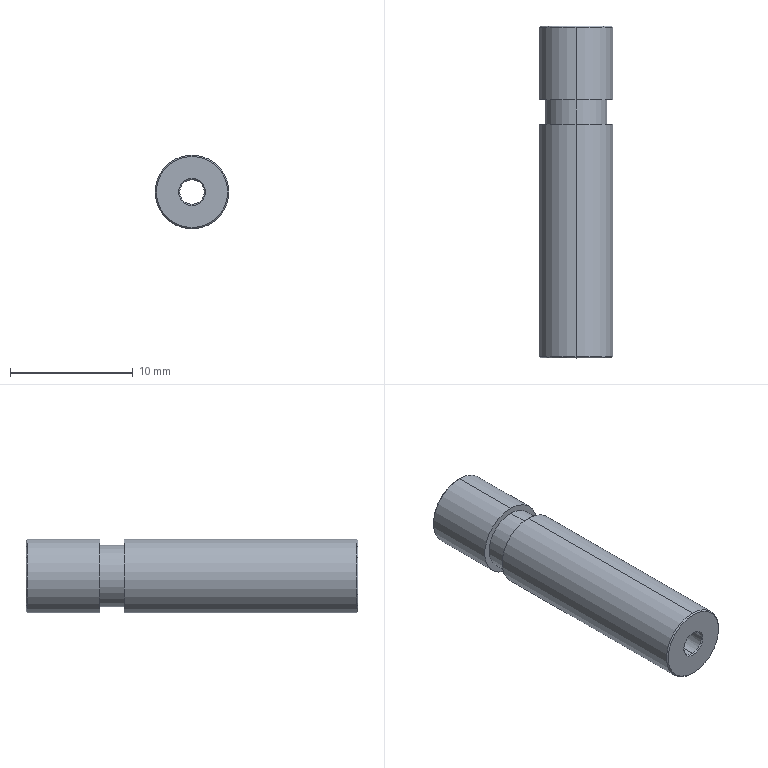Part | SolidWorks | features Revolution 1 | 1 solid | 20 faces | box 6 x 27 x 6 mm | volume 611.558 mm3 | cone 10 | cylinder 6 | plane 4 | commonest cylinder face diameters 6 x4 5 x2
STEP:
#1=CARTESIAN_POINT('',(0.,21.,-2.5));
#2=VERTEX_POINT('',#1);
#3=CARTESIAN_POINT('',(0.,21.,2.5));
#4=VERTEX_POINT('',#3);
#5=CARTESIAN_POINT('',(0.,21.,0.));
#6=DIRECTION('',(0.,-1.,0.));
#7=DIRECTION('',(0.,0.,-1.));
#8=AXIS2_PLACEMENT_3D('',#5,#6,#7);
#9=CIRCLE('',#8,2.5);
#10=EDGE_CURVE('',#2,#4,#9,.T.);
#11=ORIENTED_EDGE('',*,*,#10,.T.);
#12=CARTESIAN_POINT('',(0.,19.,2.5));
#13=VERTEX_POINT('',#12);
#14=CARTESIAN_POINT('',(0.,0.,2.5));
#15=DIRECTION('',(0.,-1.,0.));
#16=VECTOR('',#15,1000.);
#17=LINE('',#14,#16);
#18=EDGE_CURVE('',#4,#13,#17,.T.);
#19=ORIENTED_EDGE('',*,*,#18,.T.);
#20=CARTESIAN_POINT('',(0.,19.,-2.5));
#21=VERTEX_POINT('',#20);
#22=CARTESIAN_POINT('',(0.,19.,0.));
#23=DIRECTION('',(0.,-1.,0.));
#24=DIRECTION('',(0.,0.,-1.));
#25=AXIS2_PLACEMENT_3D('',#22,#23,#24);
#26=CIRCLE('',#25,2.5);
#27=EDGE_CURVE('',#21,#13,#26,.T.);
#28=ORIENTED_EDGE('',*,*,#27,.F.);
#29=CARTESIAN_POINT('',(0.,0.,-2.5));
#30=DIRECTION('',(0.,-1.,0.));
#31=VECTOR('',#30,1000.);
#32=LINE('',#29,#31);
#33=EDGE_CURVE('',#2,#21,#32,.T.);
#34=ORIENTED_EDGE('',*,*,#33,.F.);
#35=EDGE_LOOP('',(#11,#19,#28,#34));
#36=FACE_OUTER_BOUND('',#35,.T.);
#37=CARTESIAN_POINT('',(0.,0.,0.));
#38=DIRECTION('',(0.,-1.,0.));
#39=DIRECTION('',(0.,0.,-1.));
#40=AXIS2_PLACEMENT_3D('',#37,#38,#39);
#41=CYLINDRICAL_SURFACE('',#40,2.5);
#42=ADVANCED_FACE('',(#36),#41,.T.);
#43=CARTESIAN_POINT('',(0.,19.,-3.));
#44=VERTEX_POINT('',#43);
#45=CARTESIAN_POINT('',(0.,19.,3.));
#46=VERTEX_POINT('',#45);
#47=CARTESIAN_POINT('',(0.,19.,0.));
#48=DIRECTION('',(0.,-1.,0.));
#49=DIRECTION('',(0.,0.,-1.));
#50=AXIS2_PLACEMENT_3D('',#47,#48,#49);
#51=CIRCLE('',#50,3.);
#52=EDGE_CURVE('',#44,#46,#51,.T.);
#53=ORIENTED_EDGE('',*,*,#52,.T.);
#54=CARTESIAN_POINT('',(0.,0.1,3.));
#55=VERTEX_POINT('',#54);
#56=CARTESIAN_POINT('',(0.,0.,3.));
#57=DIRECTION('',(0.,-1.,0.));
#58=VECTOR('',#57,1000.);
#59=LINE('',#56,#58);
#60=EDGE_CURVE('',#46,#55,#59,.T.);
#61=ORIENTED_EDGE('',*,*,#60,.T.);
#62=CARTESIAN_POINT('',(0.,0.1,-3.));
#63=VERTEX_POINT('',#62);
#64=CARTESIAN_POINT('',(0.,0.1,0.));
#65=DIRECTION('',(0.,-1.,0.));
#66=DIRECTION('',(0.,0.,-1.));
#67=AXIS2_PLACEMENT_3D('',#64,#65,#66);
#68=CIRCLE('',#67,3.);
#69=EDGE_CURVE('',#63,#55,#68,.T.);
#70=ORIENTED_EDGE('',*,*,#69,.F.);
#71=CARTESIAN_POINT('',(0.,0.,-3.));
#72=DIRECTION('',(0.,-1.,0.));
#73=VECTOR('',#72,1000.);
#74=LINE('',#71,#73);
#75=EDGE_CURVE('',#44,#63,#74,.T.);
#76=ORIENTED_EDGE('',*,*,#75,.F.);
#77=EDGE_LOOP('',(#53,#61,#70,#76));
#78=FACE_OUTER_BOUND('',#77,.T.);
#79=CARTESIAN_POINT('',(0.,0.,0.));
#80=DIRECTION('',(0.,-1.,0.));
#81=DIRECTION('',(0.,0.,-1.));
#82=AXIS2_PLACEMENT_3D('',#79,#80,#81);
#83=CYLINDRICAL_SURFACE('',#82,3.);
#84=ADVANCED_FACE('',(#78),#83,.T.);
#85=CARTESIAN_POINT('',(0.,0.,-2.9));
#86=VERTEX_POINT('',#85);
#87=CARTESIAN_POINT('',(0.,0.,2.9));
#88=VERTEX_POINT('',#87);
#89=CARTESIAN_POINT('',(0.,0.,0.));
#90=DIRECTION('',(0.,-1.,0.));
#91=DIRECTION('',(0.,0.,-1.));
#92=AXIS2_PLACEMENT_3D('',#89,#90,#91);
#93=CIRCLE('',#92,2.9);
#94=EDGE_CURVE('',#86,#88,#93,.T.);
#95=ORIENTED_EDGE('',*,*,#94,.F.);
#96=CARTESIAN_POINT('',(0.,0.,-2.9));
#97=DIRECTION('',(0.,0.7071,-0.7071));
#98=VECTOR('',#97,1000.);
#99=LINE('',#96,#98);
#100=EDGE_CURVE('',#86,#63,#99,.T.);
#101=ORIENTED_EDGE('',*,*,#100,.T.);
#102=ORIENTED_EDGE('',*,*,#69,.T.);
#103=CARTESIAN_POINT('',(0.,0.,2.9));
#104=DIRECTION('',(0.,0.7071,0.7071));
#105=VECTOR('',#104,1000.);
#106=LINE('',#103,#105);
#107=EDGE_CURVE('',#88,#55,#106,.T.);
#108=ORIENTED_EDGE('',*,*,#107,.F.);
#109=EDGE_LOOP('',(#95,#101,#102,#108));
#110=FACE_OUTER_BOUND('',#109,.T.);
#111=CARTESIAN_POINT('',(0.,0.,0.));
#112=DIRECTION('',(0.,1.,0.));
#113=DIRECTION('',(0.,0.,1.));
#114=AXIS2_PLACEMENT_3D('',#111,#112,#113);
#115=CONICAL_SURFACE('',#114,2.9,0.7854);
#116=ADVANCED_FACE('',(#110),#115,.T.);
#117=CARTESIAN_POINT('',(0.,0.09998,1.002));
#118=VERTEX_POINT('',#117);
#119=CARTESIAN_POINT('',(0.,0.09998,-1.002));
#120=VERTEX_POINT('',#119);
#121=CARTESIAN_POINT('',(0.,0.09998,0.));
#122=DIRECTION('',(0.,-1.,0.));
#123=DIRECTION('',(0.,0.,-1.));
#124=AXIS2_PLACEMENT_3D('',#121,#122,#123);
#125=CIRCLE('',#124,1.002);
#126=EDGE_CURVE('',#118,#120,#125,.T.);
#127=ORIENTED_EDGE('',*,*,#126,.F.);
#128=CARTESIAN_POINT('',(0.,0.,1.1));
#129=VERTEX_POINT('',#128);
#130=CARTESIAN_POINT('',(0.,0.09998,1.002));
#131=DIRECTION('',(0.,-0.7136,0.7005));
#132=VECTOR('',#131,1000.);
#133=LINE('',#130,#132);
#134=EDGE_CURVE('',#118,#129,#133,.T.);
#135=ORIENTED_EDGE('',*,*,#134,.T.);
#136=CARTESIAN_POINT('',(0.,0.,-1.1));
#137=VERTEX_POINT('',#136);
#138=CARTESIAN_POINT('',(0.,0.,0.));
#139=DIRECTION('',(0.,-1.,0.));
#140=DIRECTION('',(0.,0.,-1.));
#141=AXIS2_PLACEMENT_3D('',#138,#139,#140);
#142=CIRCLE('',#141,1.1);
#143=EDGE_CURVE('',#129,#137,#142,.T.);
#144=ORIENTED_EDGE('',*,*,#143,.T.);
#145=CARTESIAN_POINT('',(0.,0.09998,-1.002));
#146=DIRECTION('',(0.,-0.7136,-0.7005));
#147=VECTOR('',#146,1000.);
#148=LINE('',#145,#147);
#149=EDGE_CURVE('',#120,#137,#148,.T.);
#150=ORIENTED_EDGE('',*,*,#149,.F.);
#151=EDGE_LOOP('',(#127,#135,#144,#150));
#152=FACE_OUTER_BOUND('',#151,.T.);
#153=CARTESIAN_POINT('',(0.,0.09998,0.));
#154=DIRECTION('',(0.,-1.,0.));
#155=DIRECTION('',(0.,0.,-1.));
#156=AXIS2_PLACEMENT_3D('',#153,#154,#155);
#157=CONICAL_SURFACE('',#156,1.002,0.7761);
#158=ADVANCED_FACE('',(#152),#157,.F.);
#159=ORIENTED_EDGE('',*,*,#126,.T.);
#160=CARTESIAN_POINT('',(0.,26.9,-1.498));
#161=VERTEX_POINT('',#160);
#162=CARTESIAN_POINT('',(0.,26.9,-1.498));
#163=DIRECTION('',(0.,0.9998,-0.01852));
#164=VECTOR('',#163,1000.);
#165=LINE('',#162,#164);
#166=EDGE_CURVE('',#120,#161,#165,.T.);
#167=ORIENTED_EDGE('',*,*,#166,.T.);
#168=CARTESIAN_POINT('',(0.,26.9,1.498));
#169=VERTEX_POINT('',#168);
#170=CARTESIAN_POINT('',(0.,26.9,0.));
#171=DIRECTION('',(0.,-1.,0.));
#172=DIRECTION('',(0.,0.,-1.));
#173=AXIS2_PLACEMENT_3D('',#170,#171,#172);
#174=CIRCLE('',#173,1.498);
#175=EDGE_CURVE('',#169,#161,#174,.T.);
#176=ORIENTED_EDGE('',*,*,#175,.F.);
#177=CARTESIAN_POINT('',(0.,26.9,1.498));
#178=DIRECTION('',(0.,0.9998,0.01852));
#179=VECTOR('',#178,1000.);
#180=LINE('',#177,#179);
#181=EDGE_CURVE('',#118,#169,#180,.T.);
#182=ORIENTED_EDGE('',*,*,#181,.F.);
#183=EDGE_LOOP('',(#159,#167,#176,#182));
#184=FACE_OUTER_BOUND('',#183,.T.);
#185=CARTESIAN_POINT('',(0.,26.9,0.));
#186=DIRECTION('',(0.,1.,0.));
#187=DIRECTION('',(0.,0.,1.));
#188=AXIS2_PLACEMENT_3D('',#185,#186,#187);
#189=CONICAL_SURFACE('',#188,1.498,0.01852);
#190=ADVANCED_FACE('',(#184),#189,.F.);
#191=ORIENTED_EDGE('',*,*,#175,.T.);
#192=CARTESIAN_POINT('',(0.,27.,-1.6));
#193=VERTEX_POINT('',#192);
#194=CARTESIAN_POINT('',(0.,27.,-1.6));
#195=DIRECTION('',(0.,0.7005,-0.7136));
#196=VECTOR('',#195,1000.);
#197=LINE('',#194,#196);
#198=EDGE_CURVE('',#161,#193,#197,.T.);
#199=ORIENTED_EDGE('',*,*,#198,.T.);
#200=CARTESIAN_POINT('',(0.,27.,1.6));
#201=VERTEX_POINT('',#200);
#202=CARTESIAN_POINT('',(0.,27.,0.));
#203=DIRECTION('',(0.,-1.,0.));
#204=DIRECTION('',(0.,0.,-1.));
#205=AXIS2_PLACEMENT_3D('',#202,#203,#204);
#206=CIRCLE('',#205,1.6);
#207=EDGE_CURVE('',#201,#193,#206,.T.);
#208=ORIENTED_EDGE('',*,*,#207,.F.);
#209=CARTESIAN_POINT('',(0.,27.,1.6));
#210=DIRECTION('',(0.,0.7005,0.7136));
#211=VECTOR('',#210,1000.);
#212=LINE('',#209,#211);
#213=EDGE_CURVE('',#169,#201,#212,.T.);
#214=ORIENTED_EDGE('',*,*,#213,.F.);
#215=EDGE_LOOP('',(#191,#199,#208,#214));
#216=FACE_OUTER_BOUND('',#215,.T.);
#217=CARTESIAN_POINT('',(0.,27.,0.));
#218=DIRECTION('',(0.,1.,0.));
#219=DIRECTION('',(0.,0.,1.));
#220=AXIS2_PLACEMENT_3D('',#217,#218,#219);
#221=CONICAL_SURFACE('',#220,1.6,0.7947);
#222=ADVANCED_FACE('',(#216),#221,.F.);
#223=CARTESIAN_POINT('',(0.,27.,-2.9));
#224=VERTEX_POINT('',#223);
#225=CARTESIAN_POINT('',(0.,27.,2.9));
#226=VERTEX_POINT('',#225);
#227=CARTESIAN_POINT('',(0.,27.,0.));
#228=DIRECTION('',(0.,-1.,0.));
#229=DIRECTION('',(0.,0.,-1.));
#230=AXIS2_PLACEMENT_3D('',#227,#228,#229);
#231=CIRCLE('',#230,2.9);
#232=EDGE_CURVE('',#224,#226,#231,.T.);
#233=ORIENTED_EDGE('',*,*,#232,.T.);
#234=CARTESIAN_POINT('',(0.,26.9,3.));
#235=VERTEX_POINT('',#234);
#236=CARTESIAN_POINT('',(0.,26.9,3.));
#237=DIRECTION('',(0.,-0.7071,0.7071));
#238=VECTOR('',#237,1000.);
#239=LINE('',#236,#238);
#240=EDGE_CURVE('',#226,#235,#239,.T.);
#241=ORIENTED_EDGE('',*,*,#240,.T.);
#242=CARTESIAN_POINT('',(0.,26.9,-3.));
#243=VERTEX_POINT('',#242);
#244=CARTESIAN_POINT('',(0.,26.9,0.));
#245=DIRECTION('',(0.,-1.,0.));
#246=DIRECTION('',(0.,0.,-1.));
#247=AXIS2_PLACEMENT_3D('',#244,#245,#246);
#248=CIRCLE('',#247,3.);
#249=EDGE_CURVE('',#243,#235,#248,.T.);
#250=ORIENTED_EDGE('',*,*,#249,.F.);
#251=CARTESIAN_POINT('',(0.,26.9,-3.));
#252=DIRECTION('',(0.,-0.7071,-0.7071));
#253=VECTOR('',#252,1000.);
#254=LINE('',#251,#253);
#255=EDGE_CURVE('',#224,#243,#254,.T.);
#256=ORIENTED_EDGE('',*,*,#255,.F.);
#257=EDGE_LOOP('',(#233,#241,#250,#256));
#258=FACE_OUTER_BOUND('',#257,.T.);
#259=CARTESIAN_POINT('',(0.,26.9,0.));
#260=DIRECTION('',(0.,-1.,0.));
#261=DIRECTION('',(0.,0.,-1.));
#262=AXIS2_PLACEMENT_3D('',#259,#260,#261);
#263=CONICAL_SURFACE('',#262,3.,0.7854);
#264=ADVANCED_FACE('',(#258),#263,.T.);
#265=ORIENTED_EDGE('',*,*,#249,.T.);
#266=CARTESIAN_POINT('',(0.,21.,3.));
#267=VERTEX_POINT('',#266);
#268=CARTESIAN_POINT('',(0.,0.,3.));
#269=DIRECTION('',(0.,-1.,0.));
#270=VECTOR('',#269,1000.);
#271=LINE('',#268,#270);
#272=EDGE_CURVE('',#235,#267,#271,.T.);
#273=ORIENTED_EDGE('',*,*,#272,.T.);
#274=CARTESIAN_POINT('',(0.,21.,-3.));
#275=VERTEX_POINT('',#274);
#276=CARTESIAN_POINT('',(0.,21.,0.));
#277=DIRECTION('',(0.,-1.,0.));
#278=DIRECTION('',(0.,0.,-1.));
#279=AXIS2_PLACEMENT_3D('',#276,#277,#278);
#280=CIRCLE('',#279,3.);
#281=EDGE_CURVE('',#275,#267,#280,.T.);
#282=ORIENTED_EDGE('',*,*,#281,.F.);
#283=CARTESIAN_POINT('',(0.,0.,-3.));
#284=DIRECTION('',(0.,-1.,0.));
#285=VECTOR('',#284,1000.);
#286=LINE('',#283,#285);
#287=EDGE_CURVE('',#243,#275,#286,.T.);
#288=ORIENTED_EDGE('',*,*,#287,.F.);
#289=EDGE_LOOP('',(#265,#273,#282,#288));
#290=FACE_OUTER_BOUND('',#289,.T.);
#291=CARTESIAN_POINT('',(0.,0.,0.));
#292=DIRECTION('',(0.,-1.,0.));
#293=DIRECTION('',(0.,0.,-1.));
#294=AXIS2_PLACEMENT_3D('',#291,#292,#293);
#295=CYLINDRICAL_SURFACE('',#294,3.);
#296=ADVANCED_FACE('',(#290),#295,.T.);
#297=ORIENTED_EDGE('',*,*,#272,.F.);
#298=CARTESIAN_POINT('',(0.,26.9,0.));
#299=DIRECTION('',(0.,-1.,0.));
#300=DIRECTION('',(0.,0.,-1.));
#301=AXIS2_PLACEMENT_3D('',#298,#299,#300);
#302=CIRCLE('',#301,3.);
#303=EDGE_CURVE('',#235,#243,#302,.T.);
#304=ORIENTED_EDGE('',*,*,#303,.T.);
#305=ORIENTED_EDGE('',*,*,#287,.T.);
#306=CARTESIAN_POINT('',(0.,21.,0.));
#307=DIRECTION('',(0.,-1.,0.));
#308=DIRECTION('',(0.,0.,-1.));
#309=AXIS2_PLACEMENT_3D('',#306,#307,#308);
#310=CIRCLE('',#309,3.);
#311=EDGE_CURVE('',#267,#275,#310,.T.);
#312=ORIENTED_EDGE('',*,*,#311,.F.);
#313=EDGE_LOOP('',(#297,#304,#305,#312));
#314=FACE_OUTER_BOUND('',#313,.T.);
#315=CARTESIAN_POINT('',(0.,0.,0.));
#316=DIRECTION('',(0.,-1.,0.));
#317=DIRECTION('',(0.,0.,-1.));
#318=AXIS2_PLACEMENT_3D('',#315,#316,#317);
#319=CYLINDRICAL_SURFACE('',#318,3.);
#320=ADVANCED_FACE('',(#314),#319,.T.);
#321=ORIENTED_EDGE('',*,*,#240,.F.);
#322=CARTESIAN_POINT('',(0.,27.,0.));
#323=DIRECTION('',(0.,-1.,0.));
#324=DIRECTION('',(0.,0.,-1.));
#325=AXIS2_PLACEMENT_3D('',#322,#323,#324);
#326=CIRCLE('',#325,2.9);
#327=EDGE_CURVE('',#226,#224,#326,.T.);
#328=ORIENTED_EDGE('',*,*,#327,.T.);
#329=ORIENTED_EDGE('',*,*,#255,.T.);
#330=ORIENTED_EDGE('',*,*,#303,.F.);
#331=EDGE_LOOP('',(#321,#328,#329,#330));
#332=FACE_OUTER_BOUND('',#331,.T.);
#333=CARTESIAN_POINT('',(0.,26.9,0.));
#334=DIRECTION('',(0.,-1.,0.));
#335=DIRECTION('',(0.,0.,-1.));
#336=AXIS2_PLACEMENT_3D('',#333,#334,#335);
#337=CONICAL_SURFACE('',#336,3.,0.7854);
#338=ADVANCED_FACE('',(#332),#337,.T.);
#339=ORIENTED_EDGE('',*,*,#207,.T.);
#340=CARTESIAN_POINT('',(0.,27.,0.));
#341=DIRECTION('',(0.,-1.,0.));
#342=DIRECTION('',(0.,0.,-1.));
#343=AXIS2_PLACEMENT_3D('',#340,#341,#342);
#344=CIRCLE('',#343,1.6);
#345=EDGE_CURVE('',#193,#201,#344,.T.);
#346=ORIENTED_EDGE('',*,*,#345,.T.);
#347=EDGE_LOOP('',(#339,#346));
#348=FACE_BOUND('',#347,.T.);
#349=ORIENTED_EDGE('',*,*,#232,.F.);
#350=ORIENTED_EDGE('',*,*,#327,.F.);
#351=EDGE_LOOP('',(#349,#350));
#352=FACE_OUTER_BOUND('',#351,.T.);
#353=CARTESIAN_POINT('',(2.9,27.,0.));
#354=DIRECTION('',(0.,1.,0.));
#355=DIRECTION('',(0.,0.,1.));
#356=AXIS2_PLACEMENT_3D('',#353,#354,#355);
#357=PLANE('',#356);
#358=ADVANCED_FACE('',(#348,#352),#357,.T.);
#359=ORIENTED_EDGE('',*,*,#198,.F.);
#360=CARTESIAN_POINT('',(0.,26.9,0.));
#361=DIRECTION('',(0.,-1.,0.));
#362=DIRECTION('',(0.,0.,-1.));
#363=AXIS2_PLACEMENT_3D('',#360,#361,#362);
#364=CIRCLE('',#363,1.498);
#365=EDGE_CURVE('',#161,#169,#364,.T.);
#366=ORIENTED_EDGE('',*,*,#365,.T.);
#367=ORIENTED_EDGE('',*,*,#213,.T.);
#368=ORIENTED_EDGE('',*,*,#345,.F.);
#369=EDGE_LOOP('',(#359,#366,#367,#368));
#370=FACE_OUTER_BOUND('',#369,.T.);
#371=CARTESIAN_POINT('',(0.,27.,0.));
#372=DIRECTION('',(0.,1.,0.));
#373=DIRECTION('',(0.,0.,1.));
#374=AXIS2_PLACEMENT_3D('',#371,#372,#373);
#375=CONICAL_SURFACE('',#374,1.6,0.7947);
#376=ADVANCED_FACE('',(#370),#375,.F.);
#377=ORIENTED_EDGE('',*,*,#166,.F.);
#378=CARTESIAN_POINT('',(0.,0.09998,0.));
#379=DIRECTION('',(0.,-1.,0.));
#380=DIRECTION('',(0.,0.,-1.));
#381=AXIS2_PLACEMENT_3D('',#378,#379,#380);
#382=CIRCLE('',#381,1.002);
#383=EDGE_CURVE('',#120,#118,#382,.T.);
#384=ORIENTED_EDGE('',*,*,#383,.T.);
#385=ORIENTED_EDGE('',*,*,#181,.T.);
#386=ORIENTED_EDGE('',*,*,#365,.F.);
#387=EDGE_LOOP('',(#377,#384,#385,#386));
#388=FACE_OUTER_BOUND('',#387,.T.);
#389=CARTESIAN_POINT('',(0.,26.9,0.));
#390=DIRECTION('',(0.,1.,0.));
#391=DIRECTION('',(0.,0.,1.));
#392=AXIS2_PLACEMENT_3D('',#389,#390,#391);
#393=CONICAL_SURFACE('',#392,1.498,0.01852);
#394=ADVANCED_FACE('',(#388),#393,.F.);
#395=ORIENTED_EDGE('',*,*,#134,.F.);
#396=ORIENTED_EDGE('',*,*,#383,.F.);
#397=ORIENTED_EDGE('',*,*,#149,.T.);
#398=CARTESIAN_POINT('',(0.,0.,0.));
#399=DIRECTION('',(0.,-1.,0.));
#400=DIRECTION('',(0.,0.,-1.));
#401=AXIS2_PLACEMENT_3D('',#398,#399,#400);
#402=CIRCLE('',#401,1.1);
#403=EDGE_CURVE('',#137,#129,#402,.T.);
#404=ORIENTED_EDGE('',*,*,#403,.T.);
#405=EDGE_LOOP('',(#395,#396,#397,#404));
#406=FACE_OUTER_BOUND('',#405,.T.);
#407=CARTESIAN_POINT('',(0.,0.09998,0.));
#408=DIRECTION('',(0.,-1.,0.));
#409=DIRECTION('',(0.,0.,-1.));
#410=AXIS2_PLACEMENT_3D('',#407,#408,#409);
#411=CONICAL_SURFACE('',#410,1.002,0.7761);
#412=ADVANCED_FACE('',(#406),#411,.F.);
#413=CARTESIAN_POINT('',(0.,0.,0.));
#414=DIRECTION('',(0.,-1.,0.));
#415=DIRECTION('',(0.,0.,-1.));
#416=AXIS2_PLACEMENT_3D('',#413,#414,#415);
#417=CIRCLE('',#416,2.9);
#418=EDGE_CURVE('',#88,#86,#417,.T.);
#419=ORIENTED_EDGE('',*,*,#418,.T.);
#420=ORIENTED_EDGE('',*,*,#94,.T.);
#421=EDGE_LOOP('',(#419,#420));
#422=FACE_OUTER_BOUND('',#421,.T.);
#423=ORIENTED_EDGE('',*,*,#403,.F.);
#424=ORIENTED_EDGE('',*,*,#143,.F.);
#425=EDGE_LOOP('',(#423,#424));
#426=FACE_BOUND('',#425,.T.);
#427=CARTESIAN_POINT('',(1.1,0.,0.));
#428=DIRECTION('',(0.,-1.,0.));
#429=DIRECTION('',(0.,0.,-1.));
#430=AXIS2_PLACEMENT_3D('',#427,#428,#429);
#431=PLANE('',#430);
#432=ADVANCED_FACE('',(#422,#426),#431,.T.);
#433=ORIENTED_EDGE('',*,*,#100,.F.);
#434=ORIENTED_EDGE('',*,*,#418,.F.);
#435=ORIENTED_EDGE('',*,*,#107,.T.);
#436=CARTESIAN_POINT('',(0.,0.1,0.));
#437=DIRECTION('',(0.,-1.,0.));
#438=DIRECTION('',(0.,0.,-1.));
#439=AXIS2_PLACEMENT_3D('',#436,#437,#438);
#440=CIRCLE('',#439,3.);
#441=EDGE_CURVE('',#55,#63,#440,.T.);
#442=ORIENTED_EDGE('',*,*,#441,.T.);
#443=EDGE_LOOP('',(#433,#434,#435,#442));
#444=FACE_OUTER_BOUND('',#443,.T.);
#445=CARTESIAN_POINT('',(0.,0.,0.));
#446=DIRECTION('',(0.,1.,0.));
#447=DIRECTION('',(0.,0.,1.));
#448=AXIS2_PLACEMENT_3D('',#445,#446,#447);
#449=CONICAL_SURFACE('',#448,2.9,0.7854);
#450=ADVANCED_FACE('',(#444),#449,.T.);
#451=ORIENTED_EDGE('',*,*,#60,.F.);
#452=CARTESIAN_POINT('',(0.,19.,0.));
#453=DIRECTION('',(0.,-1.,0.));
#454=DIRECTION('',(0.,0.,-1.));
#455=AXIS2_PLACEMENT_3D('',#452,#453,#454);
#456=CIRCLE('',#455,3.);
#457=EDGE_CURVE('',#46,#44,#456,.T.);
#458=ORIENTED_EDGE('',*,*,#457,.T.);
#459=ORIENTED_EDGE('',*,*,#75,.T.);
#460=ORIENTED_EDGE('',*,*,#441,.F.);
#461=EDGE_LOOP('',(#451,#458,#459,#460));
#462=FACE_OUTER_BOUND('',#461,.T.);
#463=CARTESIAN_POINT('',(0.,0.,0.));
#464=DIRECTION('',(0.,-1.,0.));
#465=DIRECTION('',(0.,0.,-1.));
#466=AXIS2_PLACEMENT_3D('',#463,#464,#465);
#467=CYLINDRICAL_SURFACE('',#466,3.);
#468=ADVANCED_FACE('',(#462),#467,.T.);
#469=ORIENTED_EDGE('',*,*,#27,.T.);
#470=CARTESIAN_POINT('',(0.,19.,0.));
#471=DIRECTION('',(0.,-1.,0.));
#472=DIRECTION('',(0.,0.,-1.));
#473=AXIS2_PLACEMENT_3D('',#470,#471,#472);
#474=CIRCLE('',#473,2.5);
#475=EDGE_CURVE('',#13,#21,#474,.T.);
#476=ORIENTED_EDGE('',*,*,#475,.T.);
#477=EDGE_LOOP('',(#469,#476));
#478=FACE_BOUND('',#477,.T.);
#479=ORIENTED_EDGE('',*,*,#52,.F.);
#480=ORIENTED_EDGE('',*,*,#457,.F.);
#481=EDGE_LOOP('',(#479,#480));
#482=FACE_OUTER_BOUND('',#481,.T.);
#483=CARTESIAN_POINT('',(3.,19.,0.));
#484=DIRECTION('',(0.,1.,0.));
#485=DIRECTION('',(0.,0.,1.));
#486=AXIS2_PLACEMENT_3D('',#483,#484,#485);
#487=PLANE('',#486);
#488=ADVANCED_FACE('',(#478,#482),#487,.T.);
#489=ORIENTED_EDGE('',*,*,#18,.F.);
#490=CARTESIAN_POINT('',(0.,21.,0.));
#491=DIRECTION('',(0.,-1.,0.));
#492=DIRECTION('',(0.,0.,-1.));
#493=AXIS2_PLACEMENT_3D('',#490,#491,#492);
#494=CIRCLE('',#493,2.5);
#495=EDGE_CURVE('',#4,#2,#494,.T.);
#496=ORIENTED_EDGE('',*,*,#495,.T.);
#497=ORIENTED_EDGE('',*,*,#33,.T.);
#498=ORIENTED_EDGE('',*,*,#475,.F.);
#499=EDGE_LOOP('',(#489,#496,#497,#498));
#500=FACE_OUTER_BOUND('',#499,.T.);
#501=CARTESIAN_POINT('',(0.,0.,0.));
#502=DIRECTION('',(0.,-1.,0.));
#503=DIRECTION('',(0.,0.,-1.));
#504=AXIS2_PLACEMENT_3D('',#501,#502,#503);
#505=CYLINDRICAL_SURFACE('',#504,2.5);
#506=ADVANCED_FACE('',(#500),#505,.T.);
#507=ORIENTED_EDGE('',*,*,#281,.T.);
#508=ORIENTED_EDGE('',*,*,#311,.T.);
#509=EDGE_LOOP('',(#507,#508));
#510=FACE_OUTER_BOUND('',#509,.T.);
#511=ORIENTED_EDGE('',*,*,#10,.F.);
#512=ORIENTED_EDGE('',*,*,#495,.F.);
#513=EDGE_LOOP('',(#511,#512));
#514=FACE_BOUND('',#513,.T.);
#515=CARTESIAN_POINT('',(3.,21.,0.));
#516=DIRECTION('',(0.,-1.,0.));
#517=DIRECTION('',(0.,0.,-1.));
#518=AXIS2_PLACEMENT_3D('',#515,#516,#517);
#519=PLANE('',#518);
#520=ADVANCED_FACE('',(#510,#514),#519,.T.);
#521=CLOSED_SHELL('',(#42,#84,#116,#158,#190,#222,#264,#296,#320,#338,#358,#376,#394,#412,#432,#450,#468,#488,#506,#520));
#522=MANIFOLD_SOLID_BREP('',#521);
#523=CARTESIAN_POINT('',(0.,0.,0.));
#524=DIRECTION('',(0.,0.,1.));
#525=DIRECTION('',(1.,0.,0.));
#526=AXIS2_PLACEMENT_3D('',#523,#524,#525);
#527=(LENGTH_UNIT()NAMED_UNIT(*)SI_UNIT(.MILLI.,.METRE.));
#528=UNCERTAINTY_MEASURE_WITH_UNIT(LENGTH_MEASURE(0.00001),#527,'','');
#529=(NAMED_UNIT(*)PLANE_ANGLE_UNIT()SI_UNIT($,.RADIAN.));
#530=(NAMED_UNIT(*)SI_UNIT($,.STERADIAN.)SOLID_ANGLE_UNIT());
#531=(GEOMETRIC_REPRESENTATION_CONTEXT(3)GLOBAL_UNCERTAINTY_ASSIGNED_CONTEXT((#528))GLOBAL_UNIT_ASSIGNED_CONTEXT((#527,#529,#530))REPRESENTATION_CONTEXT('',''));
#532=ADVANCED_BREP_SHAPE_REPRESENTATION('',(#522,#526),#531);